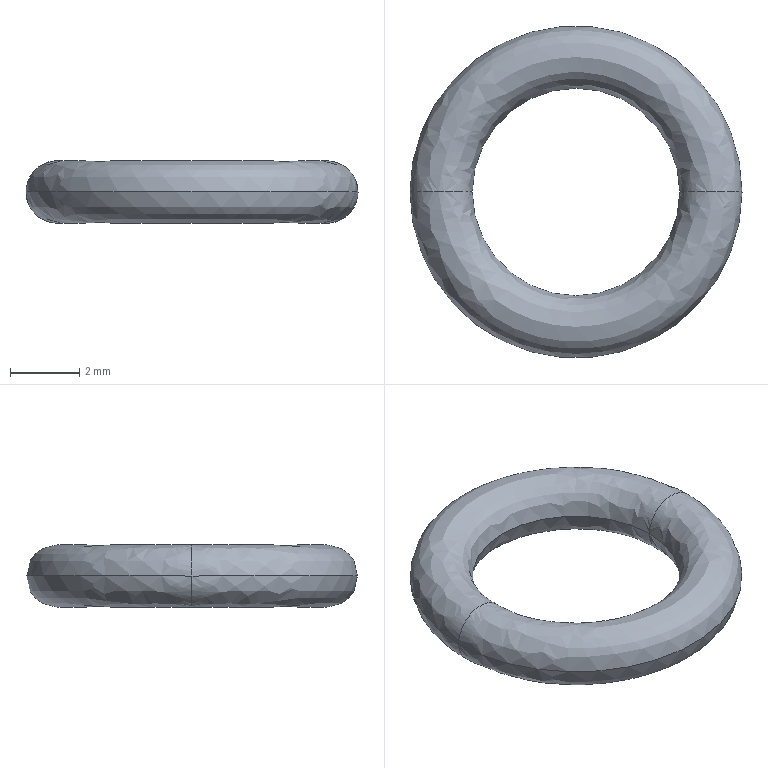Part | STEP file | Inner dia 6 wire dia 1.8 O-ring | 1 solid | 4 faces | box 9.6 x 9.6 x 1.8 mm | volume 62.351 mm3 | spline 4
STEP:
#1=CARTESIAN_POINT('',(0.,0.,0.));
#2=DIRECTION('',(0.,0.,1.));
#3=DIRECTION('',(1.,0.,0.));
#4=AXIS2_PLACEMENT_3D('',#1,#2,#3);
#5=CARTESIAN_POINT('',(4.8,0.,0.));
#6=VERTEX_POINT('',#5);
#7=CARTESIAN_POINT('',(3.,0.,0.));
#8=VERTEX_POINT('',#7);
#9=CARTESIAN_POINT('',(4.8,0.,0.));
#10=CARTESIAN_POINT('',(4.8,0.,0.5317));
#11=CARTESIAN_POINT('',(4.423,0.,0.9));
#12=CARTESIAN_POINT('',(3.9,0.,0.9));
#13=CARTESIAN_POINT('',(3.377,0.,0.9));
#14=CARTESIAN_POINT('',(3.,0.,0.5317));
#15=CARTESIAN_POINT('',(3.,0.,0.));
#16=(BOUNDED_CURVE()B_SPLINE_CURVE(3,(#9,#10,#11,#12,#13,#14,#15),.UNSPECIFIED.,.F.,.F.)B_SPLINE_CURVE_WITH_KNOTS((4,3,4),(0.03301,0.5,0.967),.UNSPECIFIED.)CURVE()GEOMETRIC_REPRESENTATION_ITEM()RATIONAL_B_SPLINE_CURVE((0.9594,0.7815,0.7951,1.,0.7951,0.7815,0.9594))REPRESENTATION_ITEM(''));
#17=CARTESIAN_POINT('',(-3.004,0.,-0.08985));
#18=CARTESIAN_POINT('',(-3.004,-6.009,-0.08985));
#19=CARTESIAN_POINT('',(3.004,-6.009,-0.08985));
#20=CARTESIAN_POINT('',(3.004,0.,-0.08985));
#21=CARTESIAN_POINT('',(-2.948,0.,0.4773));
#22=CARTESIAN_POINT('',(-2.948,-5.895,0.4773));
#23=CARTESIAN_POINT('',(2.948,-5.895,0.4773));
#24=CARTESIAN_POINT('',(2.948,0.,0.4773));
#25=CARTESIAN_POINT('',(-3.33,0.,0.9));
#26=CARTESIAN_POINT('',(-3.33,-6.66,0.9));
#27=CARTESIAN_POINT('',(3.33,-6.66,0.9));
#28=CARTESIAN_POINT('',(3.33,0.,0.9));
#29=CARTESIAN_POINT('',(-3.9,0.,0.9));
#30=CARTESIAN_POINT('',(-3.9,-7.8,0.9));
#31=CARTESIAN_POINT('',(3.9,-7.8,0.9));
#32=CARTESIAN_POINT('',(3.9,0.,0.9));
#33=CARTESIAN_POINT('',(-4.47,0.,0.9));
#34=CARTESIAN_POINT('',(-4.47,-8.94,0.9));
#35=CARTESIAN_POINT('',(4.47,-8.94,0.9));
#36=CARTESIAN_POINT('',(4.47,0.,0.9));
#37=CARTESIAN_POINT('',(-4.852,0.,0.4773));
#38=CARTESIAN_POINT('',(-4.852,-9.705,0.4773));
#39=CARTESIAN_POINT('',(4.852,-9.705,0.4773));
#40=CARTESIAN_POINT('',(4.852,0.,0.4773));
#41=CARTESIAN_POINT('',(-4.796,0.,-0.08985));
#42=CARTESIAN_POINT('',(-4.796,-9.591,-0.08985));
#43=CARTESIAN_POINT('',(4.796,-9.591,-0.08985));
#44=CARTESIAN_POINT('',(4.796,0.,-0.08985));
#45=(BOUNDED_SURFACE()B_SPLINE_SURFACE(3,3,((#17,#18,#19,#20),(#21,#22,#23,#24),(#25,#26,#27,#28),(#29,#30,#31,#32),(#33,#34,#35,#36),(#37,#38,#39,#40),(#41,#42,#43,#44)),.UNSPECIFIED.,.F.,.F.,.F.)B_SPLINE_SURFACE_WITH_KNOTS((4,3,4),(4,4),(0.,0.5,1.),(0.,1.),.PIECEWISE_BEZIER_KNOTS.)GEOMETRIC_REPRESENTATION_ITEM()RATIONAL_B_SPLINE_SURFACE(((1.,0.3333,0.3333,1.),(0.7806,0.2602,0.2602,0.7806),(0.7806,0.2602,0.2602,0.7806),(1.,0.3333,0.3333,1.),(0.7806,0.2602,0.2602,0.7806),(0.7806,0.2602,0.2602,0.7806),(1.,0.3333,0.3333,1.)))REPRESENTATION_ITEM('')SURFACE());
#46=CARTESIAN_POINT('',(1.,1.));
#47=DIRECTION('',(-1.,0.));
#48=VECTOR('',#47,1.);
#49=LINE('',#46,#48);
#50=(GEOMETRIC_REPRESENTATION_CONTEXT(2)PARAMETRIC_REPRESENTATION_CONTEXT()REPRESENTATION_CONTEXT('',''));
#51=DEFINITIONAL_REPRESENTATION('',(#49),#50);
#52=PCURVE('',#45,#51);
#53=CARTESIAN_POINT('',(3.004,0.,-0.08985));
#54=CARTESIAN_POINT('',(3.004,6.009,-0.08985));
#55=CARTESIAN_POINT('',(-3.004,6.009,-0.08985));
#56=CARTESIAN_POINT('',(-3.004,0.,-0.08985));
#57=CARTESIAN_POINT('',(2.948,0.,0.4773));
#58=CARTESIAN_POINT('',(2.948,5.895,0.4773));
#59=CARTESIAN_POINT('',(-2.948,5.895,0.4773));
#60=CARTESIAN_POINT('',(-2.948,0.,0.4773));
#61=CARTESIAN_POINT('',(3.33,0.,0.9));
#62=CARTESIAN_POINT('',(3.33,6.66,0.9));
#63=CARTESIAN_POINT('',(-3.33,6.66,0.9));
#64=CARTESIAN_POINT('',(-3.33,0.,0.9));
#65=CARTESIAN_POINT('',(3.9,0.,0.9));
#66=CARTESIAN_POINT('',(3.9,7.8,0.9));
#67=CARTESIAN_POINT('',(-3.9,7.8,0.9));
#68=CARTESIAN_POINT('',(-3.9,0.,0.9));
#69=CARTESIAN_POINT('',(4.47,0.,0.9));
#70=CARTESIAN_POINT('',(4.47,8.94,0.9));
#71=CARTESIAN_POINT('',(-4.47,8.94,0.9));
#72=CARTESIAN_POINT('',(-4.47,0.,0.9));
#73=CARTESIAN_POINT('',(4.852,0.,0.4773));
#74=CARTESIAN_POINT('',(4.852,9.705,0.4773));
#75=CARTESIAN_POINT('',(-4.852,9.705,0.4773));
#76=CARTESIAN_POINT('',(-4.852,0.,0.4773));
#77=CARTESIAN_POINT('',(4.796,0.,-0.08985));
#78=CARTESIAN_POINT('',(4.796,9.591,-0.08985));
#79=CARTESIAN_POINT('',(-4.796,9.591,-0.08985));
#80=CARTESIAN_POINT('',(-4.796,0.,-0.08985));
#81=(BOUNDED_SURFACE()B_SPLINE_SURFACE(3,3,((#53,#54,#55,#56),(#57,#58,#59,#60),(#61,#62,#63,#64),(#65,#66,#67,#68),(#69,#70,#71,#72),(#73,#74,#75,#76),(#77,#78,#79,#80)),.UNSPECIFIED.,.F.,.F.,.F.)B_SPLINE_SURFACE_WITH_KNOTS((4,3,4),(4,4),(0.,0.5,1.),(0.,1.),.PIECEWISE_BEZIER_KNOTS.)GEOMETRIC_REPRESENTATION_ITEM()RATIONAL_B_SPLINE_SURFACE(((1.,0.3333,0.3333,1.),(0.7806,0.2602,0.2602,0.7806),(0.7806,0.2602,0.2602,0.7806),(1.,0.3333,0.3333,1.),(0.7806,0.2602,0.2602,0.7806),(0.7806,0.2602,0.2602,0.7806),(1.,0.3333,0.3333,1.)))REPRESENTATION_ITEM('')SURFACE());
#82=CARTESIAN_POINT('',(1.,0.));
#83=DIRECTION('',(-1.,0.));
#84=VECTOR('',#83,1.);
#85=LINE('',#82,#84);
#86=(GEOMETRIC_REPRESENTATION_CONTEXT(2)PARAMETRIC_REPRESENTATION_CONTEXT()REPRESENTATION_CONTEXT('',''));
#87=DEFINITIONAL_REPRESENTATION('',(#85),#86);
#88=PCURVE('',#81,#87);
#89=SURFACE_CURVE('',#16,(#52,#88),.PCURVE_S1.);
#90=EDGE_CURVE('',#6,#8,#89,.T.);
#91=ORIENTED_EDGE('',*,*,#90,.T.);
#92=CARTESIAN_POINT('',(-3.,0.,0.));
#93=VERTEX_POINT('',#92);
#94=CARTESIAN_POINT('',(0.,0.,0.000000001));
#95=DIRECTION('',(0.,0.,-1.));
#96=DIRECTION('',(0.,1.,0.));
#97=AXIS2_PLACEMENT_3D('',#94,#95,#96);
#98=CIRCLE('',#97,3.);
#99=CARTESIAN_POINT('',(0.03301,1.));
#100=CARTESIAN_POINT('',(0.03301,0.9763));
#101=CARTESIAN_POINT('',(0.03301,0.9319));
#102=CARTESIAN_POINT('',(0.03301,0.8733));
#103=CARTESIAN_POINT('',(0.03301,0.8206));
#104=CARTESIAN_POINT('',(0.03301,0.7724));
#105=CARTESIAN_POINT('',(0.03301,0.7279));
#106=CARTESIAN_POINT('',(0.03301,0.6861));
#107=CARTESIAN_POINT('',(0.03301,0.6465));
#108=CARTESIAN_POINT('',(0.03301,0.6086));
#109=CARTESIAN_POINT('',(0.03301,0.5718));
#110=CARTESIAN_POINT('',(0.03301,0.5357));
#111=CARTESIAN_POINT('',(0.03301,0.5));
#112=CARTESIAN_POINT('',(0.03301,0.4643));
#113=CARTESIAN_POINT('',(0.03301,0.4282));
#114=CARTESIAN_POINT('',(0.03301,0.3914));
#115=CARTESIAN_POINT('',(0.03301,0.3535));
#116=CARTESIAN_POINT('',(0.03301,0.3139));
#117=CARTESIAN_POINT('',(0.03301,0.2721));
#118=CARTESIAN_POINT('',(0.03301,0.2276));
#119=CARTESIAN_POINT('',(0.03301,0.1794));
#120=CARTESIAN_POINT('',(0.03301,0.1267));
#121=CARTESIAN_POINT('',(0.03301,0.06805));
#122=CARTESIAN_POINT('',(0.03301,0.02375));
#123=CARTESIAN_POINT('',(0.03301,0.));
#124=B_SPLINE_CURVE_WITH_KNOTS('',3,(#99,#100,#101,#102,#103,#104,#105,#106,#107,#108,#109,#110,#111,#112,#113,#114,#115,#116,#117,#118,#119,#120,#121,#122,#123),.UNSPECIFIED.,.F.,.F.,(4,1,1,1,1,1,1,1,1,1,1,1,1,1,1,1,1,1,1,1,1,1,4),(1.571,1.714,1.856,1.999,2.142,2.285,2.428,2.57,2.713,2.856,2.999,3.142,3.284,3.427,3.57,3.713,3.856,3.998,4.141,4.284,4.427,4.57,4.712),.QUASI_UNIFORM_KNOTS.);
#125=(GEOMETRIC_REPRESENTATION_CONTEXT(2)PARAMETRIC_REPRESENTATION_CONTEXT()REPRESENTATION_CONTEXT('',''));
#126=DEFINITIONAL_REPRESENTATION('',(#124),#125);
#127=PCURVE('',#45,#126);
#128=CARTESIAN_POINT('',(-4.796,0.,0.08985));
#129=CARTESIAN_POINT('',(-4.796,-9.591,0.08985));
#130=CARTESIAN_POINT('',(4.796,-9.591,0.08985));
#131=CARTESIAN_POINT('',(4.796,0.,0.08985));
#132=CARTESIAN_POINT('',(-4.852,0.,-0.4773));
#133=CARTESIAN_POINT('',(-4.852,-9.705,-0.4773));
#134=CARTESIAN_POINT('',(4.852,-9.705,-0.4773));
#135=CARTESIAN_POINT('',(4.852,0.,-0.4773));
#136=CARTESIAN_POINT('',(-4.47,0.,-0.9));
#137=CARTESIAN_POINT('',(-4.47,-8.94,-0.9));
#138=CARTESIAN_POINT('',(4.47,-8.94,-0.9));
#139=CARTESIAN_POINT('',(4.47,0.,-0.9));
#140=CARTESIAN_POINT('',(-3.9,0.,-0.9));
#141=CARTESIAN_POINT('',(-3.9,-7.8,-0.9));
#142=CARTESIAN_POINT('',(3.9,-7.8,-0.9));
#143=CARTESIAN_POINT('',(3.9,0.,-0.9));
#144=CARTESIAN_POINT('',(-3.33,0.,-0.9));
#145=CARTESIAN_POINT('',(-3.33,-6.66,-0.9));
#146=CARTESIAN_POINT('',(3.33,-6.66,-0.9));
#147=CARTESIAN_POINT('',(3.33,0.,-0.9));
#148=CARTESIAN_POINT('',(-2.948,0.,-0.4773));
#149=CARTESIAN_POINT('',(-2.948,-5.895,-0.4773));
#150=CARTESIAN_POINT('',(2.948,-5.895,-0.4773));
#151=CARTESIAN_POINT('',(2.948,0.,-0.4773));
#152=CARTESIAN_POINT('',(-3.004,0.,0.08985));
#153=CARTESIAN_POINT('',(-3.004,-6.009,0.08985));
#154=CARTESIAN_POINT('',(3.004,-6.009,0.08985));
#155=CARTESIAN_POINT('',(3.004,0.,0.08985));
#156=(BOUNDED_SURFACE()B_SPLINE_SURFACE(3,3,((#128,#129,#130,#131),(#132,#133,#134,#135),(#136,#137,#138,#139),(#140,#141,#142,#143),(#144,#145,#146,#147),(#148,#149,#150,#151),(#152,#153,#154,#155)),.UNSPECIFIED.,.F.,.F.,.F.)B_SPLINE_SURFACE_WITH_KNOTS((4,3,4),(4,4),(0.,0.5,1.),(0.,1.),.PIECEWISE_BEZIER_KNOTS.)GEOMETRIC_REPRESENTATION_ITEM()RATIONAL_B_SPLINE_SURFACE(((1.,0.3333,0.3333,1.),(0.7806,0.2602,0.2602,0.7806),(0.7806,0.2602,0.2602,0.7806),(1.,0.3333,0.3333,1.),(0.7806,0.2602,0.2602,0.7806),(0.7806,0.2602,0.2602,0.7806),(1.,0.3333,0.3333,1.)))REPRESENTATION_ITEM('')SURFACE());
#157=CARTESIAN_POINT('',(0.967,1.));
#158=CARTESIAN_POINT('',(0.967,0.9763));
#159=CARTESIAN_POINT('',(0.967,0.9319));
#160=CARTESIAN_POINT('',(0.967,0.8733));
#161=CARTESIAN_POINT('',(0.967,0.8206));
#162=CARTESIAN_POINT('',(0.967,0.7724));
#163=CARTESIAN_POINT('',(0.967,0.7279));
#164=CARTESIAN_POINT('',(0.967,0.6861));
#165=CARTESIAN_POINT('',(0.967,0.6465));
#166=CARTESIAN_POINT('',(0.967,0.6086));
#167=CARTESIAN_POINT('',(0.967,0.5718));
#168=CARTESIAN_POINT('',(0.967,0.5357));
#169=CARTESIAN_POINT('',(0.967,0.5));
#170=CARTESIAN_POINT('',(0.967,0.4643));
#171=CARTESIAN_POINT('',(0.967,0.4282));
#172=CARTESIAN_POINT('',(0.967,0.3914));
#173=CARTESIAN_POINT('',(0.967,0.3535));
#174=CARTESIAN_POINT('',(0.967,0.3139));
#175=CARTESIAN_POINT('',(0.967,0.2721));
#176=CARTESIAN_POINT('',(0.967,0.2276));
#177=CARTESIAN_POINT('',(0.967,0.1794));
#178=CARTESIAN_POINT('',(0.967,0.1267));
#179=CARTESIAN_POINT('',(0.967,0.06805));
#180=CARTESIAN_POINT('',(0.967,0.02375));
#181=CARTESIAN_POINT('',(0.967,0.));
#182=B_SPLINE_CURVE_WITH_KNOTS('',3,(#157,#158,#159,#160,#161,#162,#163,#164,#165,#166,#167,#168,#169,#170,#171,#172,#173,#174,#175,#176,#177,#178,#179,#180,#181),.UNSPECIFIED.,.F.,.F.,(4,1,1,1,1,1,1,1,1,1,1,1,1,1,1,1,1,1,1,1,1,1,4),(1.571,1.714,1.856,1.999,2.142,2.285,2.428,2.57,2.713,2.856,2.999,3.142,3.284,3.427,3.57,3.713,3.856,3.998,4.141,4.284,4.427,4.57,4.712),.QUASI_UNIFORM_KNOTS.);
#183=(GEOMETRIC_REPRESENTATION_CONTEXT(2)PARAMETRIC_REPRESENTATION_CONTEXT()REPRESENTATION_CONTEXT('',''));
#184=DEFINITIONAL_REPRESENTATION('',(#182),#183);
#185=PCURVE('',#156,#184);
#186=SURFACE_CURVE('',#98,(#127,#185),.PCURVE_S1.);
#187=EDGE_CURVE('',#8,#93,#186,.T.);
#188=ORIENTED_EDGE('',*,*,#187,.T.);
#189=CARTESIAN_POINT('',(-4.8,0.,0.));
#190=VERTEX_POINT('',#189);
#191=CARTESIAN_POINT('',(-3.,0.,0.));
#192=CARTESIAN_POINT('',(-3.,0.,0.5317));
#193=CARTESIAN_POINT('',(-3.377,0.,0.9));
#194=CARTESIAN_POINT('',(-3.9,0.,0.9));
#195=CARTESIAN_POINT('',(-4.423,0.,0.9));
#196=CARTESIAN_POINT('',(-4.8,0.,0.5317));
#197=CARTESIAN_POINT('',(-4.8,0.,0.));
#198=(BOUNDED_CURVE()B_SPLINE_CURVE(3,(#191,#192,#193,#194,#195,#196,#197),.UNSPECIFIED.,.F.,.F.)B_SPLINE_CURVE_WITH_KNOTS((4,3,4),(0.03301,0.5,0.967),.PIECEWISE_BEZIER_KNOTS.)CURVE()GEOMETRIC_REPRESENTATION_ITEM()RATIONAL_B_SPLINE_CURVE((0.9594,0.7815,0.7951,1.,0.7951,0.7815,0.9594))REPRESENTATION_ITEM(''));
#199=CARTESIAN_POINT('',(0.,0.));
#200=DIRECTION('',(1.,0.));
#201=VECTOR('',#200,1.);
#202=LINE('',#199,#201);
#203=(GEOMETRIC_REPRESENTATION_CONTEXT(2)PARAMETRIC_REPRESENTATION_CONTEXT()REPRESENTATION_CONTEXT('',''));
#204=DEFINITIONAL_REPRESENTATION('',(#202),#203);
#205=PCURVE('',#45,#204);
#206=CARTESIAN_POINT('',(0.,1.));
#207=DIRECTION('',(1.,0.));
#208=VECTOR('',#207,1.);
#209=LINE('',#206,#208);
#210=(GEOMETRIC_REPRESENTATION_CONTEXT(2)PARAMETRIC_REPRESENTATION_CONTEXT()REPRESENTATION_CONTEXT('',''));
#211=DEFINITIONAL_REPRESENTATION('',(#209),#210);
#212=PCURVE('',#81,#211);
#213=SURFACE_CURVE('',#198,(#205,#212),.PCURVE_S1.);
#214=EDGE_CURVE('',#93,#190,#213,.T.);
#215=ORIENTED_EDGE('',*,*,#214,.T.);
#216=CARTESIAN_POINT('',(0.,0.,0.000000001));
#217=DIRECTION('',(0.,0.,1.));
#218=DIRECTION('',(0.,-1.,0.));
#219=AXIS2_PLACEMENT_3D('',#216,#217,#218);
#220=CIRCLE('',#219,4.8);
#221=CARTESIAN_POINT('',(0.967,0.));
#222=CARTESIAN_POINT('',(0.967,0.02375));
#223=CARTESIAN_POINT('',(0.967,0.06805));
#224=CARTESIAN_POINT('',(0.967,0.1267));
#225=CARTESIAN_POINT('',(0.967,0.1794));
#226=CARTESIAN_POINT('',(0.967,0.2276));
#227=CARTESIAN_POINT('',(0.967,0.2721));
#228=CARTESIAN_POINT('',(0.967,0.3139));
#229=CARTESIAN_POINT('',(0.967,0.3535));
#230=CARTESIAN_POINT('',(0.967,0.3914));
#231=CARTESIAN_POINT('',(0.967,0.4282));
#232=CARTESIAN_POINT('',(0.967,0.4643));
#233=CARTESIAN_POINT('',(0.967,0.5));
#234=CARTESIAN_POINT('',(0.967,0.5357));
#235=CARTESIAN_POINT('',(0.967,0.5718));
#236=CARTESIAN_POINT('',(0.967,0.6086));
#237=CARTESIAN_POINT('',(0.967,0.6465));
#238=CARTESIAN_POINT('',(0.967,0.6861));
#239=CARTESIAN_POINT('',(0.967,0.7279));
#240=CARTESIAN_POINT('',(0.967,0.7724));
#241=CARTESIAN_POINT('',(0.967,0.8206));
#242=CARTESIAN_POINT('',(0.967,0.8733));
#243=CARTESIAN_POINT('',(0.967,0.9319));
#244=CARTESIAN_POINT('',(0.967,0.9763));
#245=CARTESIAN_POINT('',(0.967,1.));
#246=B_SPLINE_CURVE_WITH_KNOTS('',3,(#221,#222,#223,#224,#225,#226,#227,#228,#229,#230,#231,#232,#233,#234,#235,#236,#237,#238,#239,#240,#241,#242,#243,#244,#245),.UNSPECIFIED.,.F.,.F.,(4,1,1,1,1,1,1,1,1,1,1,1,1,1,1,1,1,1,1,1,1,1,4),(4.712,4.855,4.998,5.141,5.284,5.426,5.569,5.712,5.855,5.998,6.14,6.283,6.426,6.569,6.712,6.854,6.997,7.14,7.283,7.426,7.568,7.711,7.854),.QUASI_UNIFORM_KNOTS.);
#247=(GEOMETRIC_REPRESENTATION_CONTEXT(2)PARAMETRIC_REPRESENTATION_CONTEXT()REPRESENTATION_CONTEXT('',''));
#248=DEFINITIONAL_REPRESENTATION('',(#246),#247);
#249=PCURVE('',#45,#248);
#250=CARTESIAN_POINT('',(0.03301,0.));
#251=CARTESIAN_POINT('',(0.03301,0.02375));
#252=CARTESIAN_POINT('',(0.03301,0.06805));
#253=CARTESIAN_POINT('',(0.03301,0.1267));
#254=CARTESIAN_POINT('',(0.03301,0.1794));
#255=CARTESIAN_POINT('',(0.03301,0.2276));
#256=CARTESIAN_POINT('',(0.03301,0.2721));
#257=CARTESIAN_POINT('',(0.03301,0.3139));
#258=CARTESIAN_POINT('',(0.03301,0.3535));
#259=CARTESIAN_POINT('',(0.03301,0.3914));
#260=CARTESIAN_POINT('',(0.03301,0.4282));
#261=CARTESIAN_POINT('',(0.03301,0.4643));
#262=CARTESIAN_POINT('',(0.03301,0.5));
#263=CARTESIAN_POINT('',(0.03301,0.5357));
#264=CARTESIAN_POINT('',(0.03301,0.5718));
#265=CARTESIAN_POINT('',(0.03301,0.6086));
#266=CARTESIAN_POINT('',(0.03301,0.6465));
#267=CARTESIAN_POINT('',(0.03301,0.6861));
#268=CARTESIAN_POINT('',(0.03301,0.7279));
#269=CARTESIAN_POINT('',(0.03301,0.7724));
#270=CARTESIAN_POINT('',(0.03301,0.8206));
#271=CARTESIAN_POINT('',(0.03301,0.8733));
#272=CARTESIAN_POINT('',(0.03301,0.9319));
#273=CARTESIAN_POINT('',(0.03301,0.9763));
#274=CARTESIAN_POINT('',(0.03301,1.));
#275=B_SPLINE_CURVE_WITH_KNOTS('',3,(#250,#251,#252,#253,#254,#255,#256,#257,#258,#259,#260,#261,#262,#263,#264,#265,#266,#267,#268,#269,#270,#271,#272,#273,#274),.UNSPECIFIED.,.F.,.F.,(4,1,1,1,1,1,1,1,1,1,1,1,1,1,1,1,1,1,1,1,1,1,4),(4.712,4.855,4.998,5.141,5.284,5.426,5.569,5.712,5.855,5.998,6.14,6.283,6.426,6.569,6.712,6.854,6.997,7.14,7.283,7.426,7.568,7.711,7.854),.QUASI_UNIFORM_KNOTS.);
#276=(GEOMETRIC_REPRESENTATION_CONTEXT(2)PARAMETRIC_REPRESENTATION_CONTEXT()REPRESENTATION_CONTEXT('',''));
#277=DEFINITIONAL_REPRESENTATION('',(#275),#276);
#278=PCURVE('',#156,#277);
#279=SURFACE_CURVE('',#220,(#249,#278),.PCURVE_S1.);
#280=EDGE_CURVE('',#190,#6,#279,.T.);
#281=ORIENTED_EDGE('',*,*,#280,.T.);
#282=EDGE_LOOP('',(#91,#188,#215,#281));
#283=FACE_BOUND('',#282,.T.);
#284=ADVANCED_FACE('',(#283),#45,.T.);
#285=ORIENTED_EDGE('',*,*,#187,.F.);
#286=CARTESIAN_POINT('',(3.,0.,0.));
#287=CARTESIAN_POINT('',(3.,0.,-0.5317));
#288=CARTESIAN_POINT('',(3.377,0.,-0.9));
#289=CARTESIAN_POINT('',(3.9,0.,-0.9));
#290=CARTESIAN_POINT('',(4.423,0.,-0.9));
#291=CARTESIAN_POINT('',(4.8,0.,-0.5317));
#292=CARTESIAN_POINT('',(4.8,0.,0.));
#293=(BOUNDED_CURVE()B_SPLINE_CURVE(3,(#286,#287,#288,#289,#290,#291,#292),.UNSPECIFIED.,.F.,.F.)B_SPLINE_CURVE_WITH_KNOTS((4,3,4),(0.03301,0.5,0.967),.UNSPECIFIED.)CURVE()GEOMETRIC_REPRESENTATION_ITEM()RATIONAL_B_SPLINE_CURVE((0.9594,0.7815,0.7951,1.,0.7951,0.7815,0.9594))REPRESENTATION_ITEM(''));
#294=CARTESIAN_POINT('',(1.,1.));
#295=DIRECTION('',(-1.,0.));
#296=VECTOR('',#295,1.);
#297=LINE('',#294,#296);
#298=(GEOMETRIC_REPRESENTATION_CONTEXT(2)PARAMETRIC_REPRESENTATION_CONTEXT()REPRESENTATION_CONTEXT('',''));
#299=DEFINITIONAL_REPRESENTATION('',(#297),#298);
#300=PCURVE('',#156,#299);
#301=CARTESIAN_POINT('',(4.796,0.,0.08985));
#302=CARTESIAN_POINT('',(4.796,9.591,0.08985));
#303=CARTESIAN_POINT('',(-4.796,9.591,0.08985));
#304=CARTESIAN_POINT('',(-4.796,0.,0.08985));
#305=CARTESIAN_POINT('',(4.852,0.,-0.4773));
#306=CARTESIAN_POINT('',(4.852,9.705,-0.4773));
#307=CARTESIAN_POINT('',(-4.852,9.705,-0.4773));
#308=CARTESIAN_POINT('',(-4.852,0.,-0.4773));
#309=CARTESIAN_POINT('',(4.47,0.,-0.9));
#310=CARTESIAN_POINT('',(4.47,8.94,-0.9));
#311=CARTESIAN_POINT('',(-4.47,8.94,-0.9));
#312=CARTESIAN_POINT('',(-4.47,0.,-0.9));
#313=CARTESIAN_POINT('',(3.9,0.,-0.9));
#314=CARTESIAN_POINT('',(3.9,7.8,-0.9));
#315=CARTESIAN_POINT('',(-3.9,7.8,-0.9));
#316=CARTESIAN_POINT('',(-3.9,0.,-0.9));
#317=CARTESIAN_POINT('',(3.33,0.,-0.9));
#318=CARTESIAN_POINT('',(3.33,6.66,-0.9));
#319=CARTESIAN_POINT('',(-3.33,6.66,-0.9));
#320=CARTESIAN_POINT('',(-3.33,0.,-0.9));
#321=CARTESIAN_POINT('',(2.948,0.,-0.4773));
#322=CARTESIAN_POINT('',(2.948,5.895,-0.4773));
#323=CARTESIAN_POINT('',(-2.948,5.895,-0.4773));
#324=CARTESIAN_POINT('',(-2.948,0.,-0.4773));
#325=CARTESIAN_POINT('',(3.004,0.,0.08985));
#326=CARTESIAN_POINT('',(3.004,6.009,0.08985));
#327=CARTESIAN_POINT('',(-3.004,6.009,0.08985));
#328=CARTESIAN_POINT('',(-3.004,0.,0.08985));
#329=(BOUNDED_SURFACE()B_SPLINE_SURFACE(3,3,((#301,#302,#303,#304),(#305,#306,#307,#308),(#309,#310,#311,#312),(#313,#314,#315,#316),(#317,#318,#319,#320),(#321,#322,#323,#324),(#325,#326,#327,#328)),.UNSPECIFIED.,.F.,.F.,.F.)B_SPLINE_SURFACE_WITH_KNOTS((4,3,4),(4,4),(0.,0.5,1.),(0.,1.),.PIECEWISE_BEZIER_KNOTS.)GEOMETRIC_REPRESENTATION_ITEM()RATIONAL_B_SPLINE_SURFACE(((1.,0.3333,0.3333,1.),(0.7806,0.2602,0.2602,0.7806),(0.7806,0.2602,0.2602,0.7806),(1.,0.3333,0.3333,1.),(0.7806,0.2602,0.2602,0.7806),(0.7806,0.2602,0.2602,0.7806),(1.,0.3333,0.3333,1.)))REPRESENTATION_ITEM('')SURFACE());
#330=CARTESIAN_POINT('',(1.,0.));
#331=DIRECTION('',(-1.,0.));
#332=VECTOR('',#331,1.);
#333=LINE('',#330,#332);
#334=(GEOMETRIC_REPRESENTATION_CONTEXT(2)PARAMETRIC_REPRESENTATION_CONTEXT()REPRESENTATION_CONTEXT('',''));
#335=DEFINITIONAL_REPRESENTATION('',(#333),#334);
#336=PCURVE('',#329,#335);
#337=SURFACE_CURVE('',#293,(#300,#336),.PCURVE_S1.);
#338=EDGE_CURVE('',#8,#6,#337,.T.);
#339=ORIENTED_EDGE('',*,*,#338,.T.);
#340=ORIENTED_EDGE('',*,*,#280,.F.);
#341=CARTESIAN_POINT('',(-4.8,0.,0.));
#342=CARTESIAN_POINT('',(-4.8,0.,-0.5317));
#343=CARTESIAN_POINT('',(-4.423,0.,-0.9));
#344=CARTESIAN_POINT('',(-3.9,0.,-0.9));
#345=CARTESIAN_POINT('',(-3.377,0.,-0.9));
#346=CARTESIAN_POINT('',(-3.,0.,-0.5317));
#347=CARTESIAN_POINT('',(-3.,0.,0.));
#348=(BOUNDED_CURVE()B_SPLINE_CURVE(3,(#341,#342,#343,#344,#345,#346,#347),.UNSPECIFIED.,.F.,.F.)B_SPLINE_CURVE_WITH_KNOTS((4,3,4),(0.03301,0.5,0.967),.PIECEWISE_BEZIER_KNOTS.)CURVE()GEOMETRIC_REPRESENTATION_ITEM()RATIONAL_B_SPLINE_CURVE((0.9594,0.7815,0.7951,1.,0.7951,0.7815,0.9594))REPRESENTATION_ITEM(''));
#349=CARTESIAN_POINT('',(0.,0.));
#350=DIRECTION('',(1.,0.));
#351=VECTOR('',#350,1.);
#352=LINE('',#349,#351);
#353=(GEOMETRIC_REPRESENTATION_CONTEXT(2)PARAMETRIC_REPRESENTATION_CONTEXT()REPRESENTATION_CONTEXT('',''));
#354=DEFINITIONAL_REPRESENTATION('',(#352),#353);
#355=PCURVE('',#156,#354);
#356=CARTESIAN_POINT('',(0.,1.));
#357=DIRECTION('',(1.,0.));
#358=VECTOR('',#357,1.);
#359=LINE('',#356,#358);
#360=(GEOMETRIC_REPRESENTATION_CONTEXT(2)PARAMETRIC_REPRESENTATION_CONTEXT()REPRESENTATION_CONTEXT('',''));
#361=DEFINITIONAL_REPRESENTATION('',(#359),#360);
#362=PCURVE('',#329,#361);
#363=SURFACE_CURVE('',#348,(#355,#362),.PCURVE_S1.);
#364=EDGE_CURVE('',#190,#93,#363,.T.);
#365=ORIENTED_EDGE('',*,*,#364,.T.);
#366=EDGE_LOOP('',(#285,#339,#340,#365));
#367=FACE_BOUND('',#366,.T.);
#368=ADVANCED_FACE('',(#367),#156,.T.);
#369=ORIENTED_EDGE('',*,*,#214,.F.);
#370=CARTESIAN_POINT('',(0.,0.,0.000000001));
#371=DIRECTION('',(0.,0.,-1.));
#372=DIRECTION('',(0.,1.,0.));
#373=AXIS2_PLACEMENT_3D('',#370,#371,#372);
#374=CIRCLE('',#373,3.);
#375=CARTESIAN_POINT('',(0.03301,1.));
#376=CARTESIAN_POINT('',(0.03301,0.9763));
#377=CARTESIAN_POINT('',(0.03301,0.9319));
#378=CARTESIAN_POINT('',(0.03301,0.8733));
#379=CARTESIAN_POINT('',(0.03301,0.8206));
#380=CARTESIAN_POINT('',(0.03301,0.7724));
#381=CARTESIAN_POINT('',(0.03301,0.7279));
#382=CARTESIAN_POINT('',(0.03301,0.6861));
#383=CARTESIAN_POINT('',(0.03301,0.6465));
#384=CARTESIAN_POINT('',(0.03301,0.6086));
#385=CARTESIAN_POINT('',(0.03301,0.5718));
#386=CARTESIAN_POINT('',(0.03301,0.5357));
#387=CARTESIAN_POINT('',(0.03301,0.5));
#388=CARTESIAN_POINT('',(0.03301,0.4643));
#389=CARTESIAN_POINT('',(0.03301,0.4282));
#390=CARTESIAN_POINT('',(0.03301,0.3914));
#391=CARTESIAN_POINT('',(0.03301,0.3535));
#392=CARTESIAN_POINT('',(0.03301,0.3139));
#393=CARTESIAN_POINT('',(0.03301,0.2721));
#394=CARTESIAN_POINT('',(0.03301,0.2276));
#395=CARTESIAN_POINT('',(0.03301,0.1794));
#396=CARTESIAN_POINT('',(0.03301,0.1267));
#397=CARTESIAN_POINT('',(0.03301,0.06805));
#398=CARTESIAN_POINT('',(0.03301,0.02375));
#399=CARTESIAN_POINT('',(0.03301,0.));
#400=B_SPLINE_CURVE_WITH_KNOTS('',3,(#375,#376,#377,#378,#379,#380,#381,#382,#383,#384,#385,#386,#387,#388,#389,#390,#391,#392,#393,#394,#395,#396,#397,#398,#399),.UNSPECIFIED.,.F.,.F.,(4,1,1,1,1,1,1,1,1,1,1,1,1,1,1,1,1,1,1,1,1,1,4),(4.712,4.855,4.998,5.141,5.284,5.426,5.569,5.712,5.855,5.998,6.14,6.283,6.426,6.569,6.712,6.854,6.997,7.14,7.283,7.426,7.568,7.711,7.854),.QUASI_UNIFORM_KNOTS.);
#401=(GEOMETRIC_REPRESENTATION_CONTEXT(2)PARAMETRIC_REPRESENTATION_CONTEXT()REPRESENTATION_CONTEXT('',''));
#402=DEFINITIONAL_REPRESENTATION('',(#400),#401);
#403=PCURVE('',#81,#402);
#404=CARTESIAN_POINT('',(0.967,1.));
#405=CARTESIAN_POINT('',(0.967,0.9763));
#406=CARTESIAN_POINT('',(0.967,0.9319));
#407=CARTESIAN_POINT('',(0.967,0.8733));
#408=CARTESIAN_POINT('',(0.967,0.8206));
#409=CARTESIAN_POINT('',(0.967,0.7724));
#410=CARTESIAN_POINT('',(0.967,0.7279));
#411=CARTESIAN_POINT('',(0.967,0.6861));
#412=CARTESIAN_POINT('',(0.967,0.6465));
#413=CARTESIAN_POINT('',(0.967,0.6086));
#414=CARTESIAN_POINT('',(0.967,0.5718));
#415=CARTESIAN_POINT('',(0.967,0.5357));
#416=CARTESIAN_POINT('',(0.967,0.5));
#417=CARTESIAN_POINT('',(0.967,0.4643));
#418=CARTESIAN_POINT('',(0.967,0.4282));
#419=CARTESIAN_POINT('',(0.967,0.3914));
#420=CARTESIAN_POINT('',(0.967,0.3535));
#421=CARTESIAN_POINT('',(0.967,0.3139));
#422=CARTESIAN_POINT('',(0.967,0.2721));
#423=CARTESIAN_POINT('',(0.967,0.2276));
#424=CARTESIAN_POINT('',(0.967,0.1794));
#425=CARTESIAN_POINT('',(0.967,0.1267));
#426=CARTESIAN_POINT('',(0.967,0.06805));
#427=CARTESIAN_POINT('',(0.967,0.02375));
#428=CARTESIAN_POINT('',(0.967,0.));
#429=B_SPLINE_CURVE_WITH_KNOTS('',3,(#404,#405,#406,#407,#408,#409,#410,#411,#412,#413,#414,#415,#416,#417,#418,#419,#420,#421,#422,#423,#424,#425,#426,#427,#428),.UNSPECIFIED.,.F.,.F.,(4,1,1,1,1,1,1,1,1,1,1,1,1,1,1,1,1,1,1,1,1,1,4),(4.712,4.855,4.998,5.141,5.284,5.426,5.569,5.712,5.855,5.998,6.14,6.283,6.426,6.569,6.712,6.854,6.997,7.14,7.283,7.426,7.568,7.711,7.854),.QUASI_UNIFORM_KNOTS.);
#430=(GEOMETRIC_REPRESENTATION_CONTEXT(2)PARAMETRIC_REPRESENTATION_CONTEXT()REPRESENTATION_CONTEXT('',''));
#431=DEFINITIONAL_REPRESENTATION('',(#429),#430);
#432=PCURVE('',#329,#431);
#433=SURFACE_CURVE('',#374,(#403,#432),.PCURVE_S1.);
#434=EDGE_CURVE('',#93,#8,#433,.T.);
#435=ORIENTED_EDGE('',*,*,#434,.T.);
#436=ORIENTED_EDGE('',*,*,#90,.F.);
#437=CARTESIAN_POINT('',(0.,0.,0.000000001));
#438=DIRECTION('',(0.,0.,1.));
#439=DIRECTION('',(0.,-1.,0.));
#440=AXIS2_PLACEMENT_3D('',#437,#438,#439);
#441=CIRCLE('',#440,4.8);
#442=CARTESIAN_POINT('',(0.967,0.));
#443=CARTESIAN_POINT('',(0.967,0.02375));
#444=CARTESIAN_POINT('',(0.967,0.06805));
#445=CARTESIAN_POINT('',(0.967,0.1267));
#446=CARTESIAN_POINT('',(0.967,0.1794));
#447=CARTESIAN_POINT('',(0.967,0.2276));
#448=CARTESIAN_POINT('',(0.967,0.2721));
#449=CARTESIAN_POINT('',(0.967,0.3139));
#450=CARTESIAN_POINT('',(0.967,0.3535));
#451=CARTESIAN_POINT('',(0.967,0.3914));
#452=CARTESIAN_POINT('',(0.967,0.4282));
#453=CARTESIAN_POINT('',(0.967,0.4643));
#454=CARTESIAN_POINT('',(0.967,0.5));
#455=CARTESIAN_POINT('',(0.967,0.5357));
#456=CARTESIAN_POINT('',(0.967,0.5718));
#457=CARTESIAN_POINT('',(0.967,0.6086));
#458=CARTESIAN_POINT('',(0.967,0.6465));
#459=CARTESIAN_POINT('',(0.967,0.6861));
#460=CARTESIAN_POINT('',(0.967,0.7279));
#461=CARTESIAN_POINT('',(0.967,0.7724));
#462=CARTESIAN_POINT('',(0.967,0.8206));
#463=CARTESIAN_POINT('',(0.967,0.8733));
#464=CARTESIAN_POINT('',(0.967,0.9319));
#465=CARTESIAN_POINT('',(0.967,0.9763));
#466=CARTESIAN_POINT('',(0.967,1.));
#467=B_SPLINE_CURVE_WITH_KNOTS('',3,(#442,#443,#444,#445,#446,#447,#448,#449,#450,#451,#452,#453,#454,#455,#456,#457,#458,#459,#460,#461,#462,#463,#464,#465,#466),.UNSPECIFIED.,.F.,.F.,(4,1,1,1,1,1,1,1,1,1,1,1,1,1,1,1,1,1,1,1,1,1,4),(1.571,1.714,1.856,1.999,2.142,2.285,2.428,2.57,2.713,2.856,2.999,3.142,3.284,3.427,3.57,3.713,3.856,3.998,4.141,4.284,4.427,4.57,4.712),.QUASI_UNIFORM_KNOTS.);
#468=(GEOMETRIC_REPRESENTATION_CONTEXT(2)PARAMETRIC_REPRESENTATION_CONTEXT()REPRESENTATION_CONTEXT('',''));
#469=DEFINITIONAL_REPRESENTATION('',(#467),#468);
#470=PCURVE('',#81,#469);
#471=CARTESIAN_POINT('',(0.03301,0.));
#472=CARTESIAN_POINT('',(0.03301,0.02375));
#473=CARTESIAN_POINT('',(0.03301,0.06805));
#474=CARTESIAN_POINT('',(0.03301,0.1267));
#475=CARTESIAN_POINT('',(0.03301,0.1794));
#476=CARTESIAN_POINT('',(0.03301,0.2276));
#477=CARTESIAN_POINT('',(0.03301,0.2721));
#478=CARTESIAN_POINT('',(0.03301,0.3139));
#479=CARTESIAN_POINT('',(0.03301,0.3535));
#480=CARTESIAN_POINT('',(0.03301,0.3914));
#481=CARTESIAN_POINT('',(0.03301,0.4282));
#482=CARTESIAN_POINT('',(0.03301,0.4643));
#483=CARTESIAN_POINT('',(0.03301,0.5));
#484=CARTESIAN_POINT('',(0.03301,0.5357));
#485=CARTESIAN_POINT('',(0.03301,0.5718));
#486=CARTESIAN_POINT('',(0.03301,0.6086));
#487=CARTESIAN_POINT('',(0.03301,0.6465));
#488=CARTESIAN_POINT('',(0.03301,0.6861));
#489=CARTESIAN_POINT('',(0.03301,0.7279));
#490=CARTESIAN_POINT('',(0.03301,0.7724));
#491=CARTESIAN_POINT('',(0.03301,0.8206));
#492=CARTESIAN_POINT('',(0.03301,0.8733));
#493=CARTESIAN_POINT('',(0.03301,0.9319));
#494=CARTESIAN_POINT('',(0.03301,0.9763));
#495=CARTESIAN_POINT('',(0.03301,1.));
#496=B_SPLINE_CURVE_WITH_KNOTS('',3,(#471,#472,#473,#474,#475,#476,#477,#478,#479,#480,#481,#482,#483,#484,#485,#486,#487,#488,#489,#490,#491,#492,#493,#494,#495),.UNSPECIFIED.,.F.,.F.,(4,1,1,1,1,1,1,1,1,1,1,1,1,1,1,1,1,1,1,1,1,1,4),(1.571,1.714,1.856,1.999,2.142,2.285,2.428,2.57,2.713,2.856,2.999,3.142,3.284,3.427,3.57,3.713,3.856,3.998,4.141,4.284,4.427,4.57,4.712),.QUASI_UNIFORM_KNOTS.);
#497=(GEOMETRIC_REPRESENTATION_CONTEXT(2)PARAMETRIC_REPRESENTATION_CONTEXT()REPRESENTATION_CONTEXT('',''));
#498=DEFINITIONAL_REPRESENTATION('',(#496),#497);
#499=PCURVE('',#329,#498);
#500=SURFACE_CURVE('',#441,(#470,#499),.PCURVE_S1.);
#501=EDGE_CURVE('',#6,#190,#500,.T.);
#502=ORIENTED_EDGE('',*,*,#501,.T.);
#503=EDGE_LOOP('',(#369,#435,#436,#502));
#504=FACE_BOUND('',#503,.T.);
#505=ADVANCED_FACE('',(#504),#81,.T.);
#506=ORIENTED_EDGE('',*,*,#434,.F.);
#507=ORIENTED_EDGE('',*,*,#364,.F.);
#508=ORIENTED_EDGE('',*,*,#501,.F.);
#509=ORIENTED_EDGE('',*,*,#338,.F.);
#510=EDGE_LOOP('',(#506,#507,#508,#509));
#511=FACE_BOUND('',#510,.T.);
#512=ADVANCED_FACE('',(#511),#329,.T.);
#513=CLOSED_SHELL('',(#284,#368,#505,#512));
#514=MANIFOLD_SOLID_BREP('',#513);
#515=(LENGTH_UNIT()NAMED_UNIT(*)SI_UNIT(.MILLI.,.METRE.));
#516=UNCERTAINTY_MEASURE_WITH_UNIT(LENGTH_MEASURE(0.0000001),#515,'','');
#517=(NAMED_UNIT(*)PLANE_ANGLE_UNIT()SI_UNIT($,.RADIAN.));
#518=(NAMED_UNIT(*)SI_UNIT($,.STERADIAN.)SOLID_ANGLE_UNIT());
#519=(GEOMETRIC_REPRESENTATION_CONTEXT(3)GLOBAL_UNCERTAINTY_ASSIGNED_CONTEXT((#516))GLOBAL_UNIT_ASSIGNED_CONTEXT((#515,#517,#518))REPRESENTATION_CONTEXT('',''));
#520=ADVANCED_BREP_SHAPE_REPRESENTATION('',(#4,#514),#519);